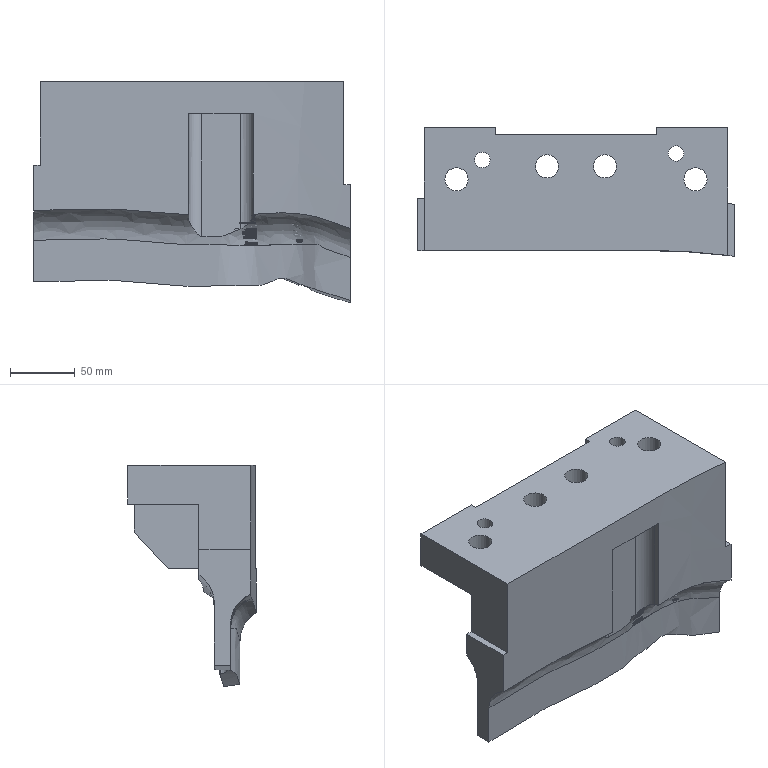Part | NX | features solid 2 | 1 solid | 65 faces | box 245.152 x 99.377 x 171.3 mm | volume 1359759 mm3 | plane 34 | spline 18 | cylinder 13 | commonest cylinder face diameters 18 x4 26 x4 12 x2 20 x2 10 x1